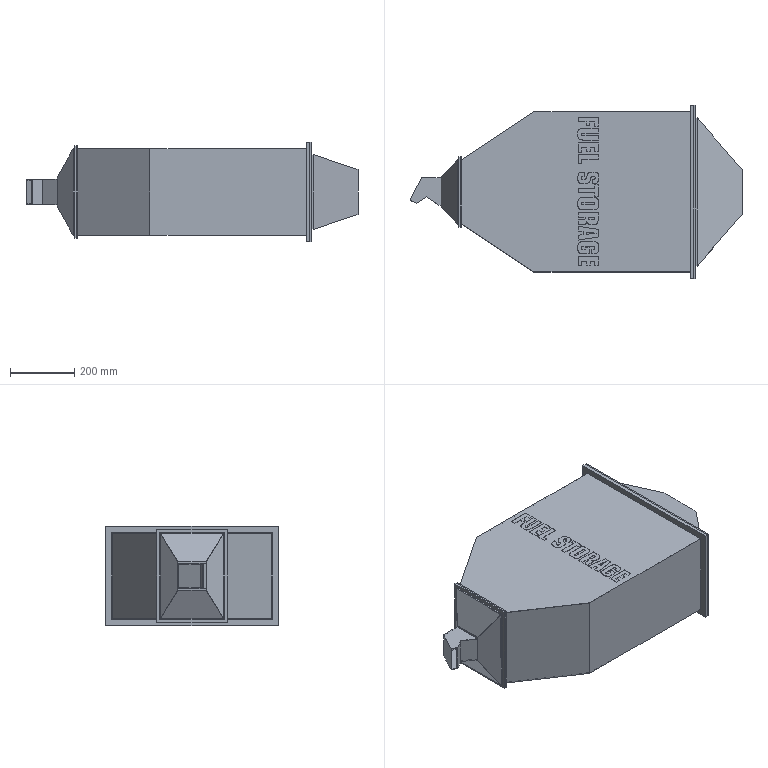Part | STEP file | Coal Storage | 14 solids | 441 faces | box 1037 x 540 x 310 mm | volume 5068760 mm3 | plane 337 | spline 104